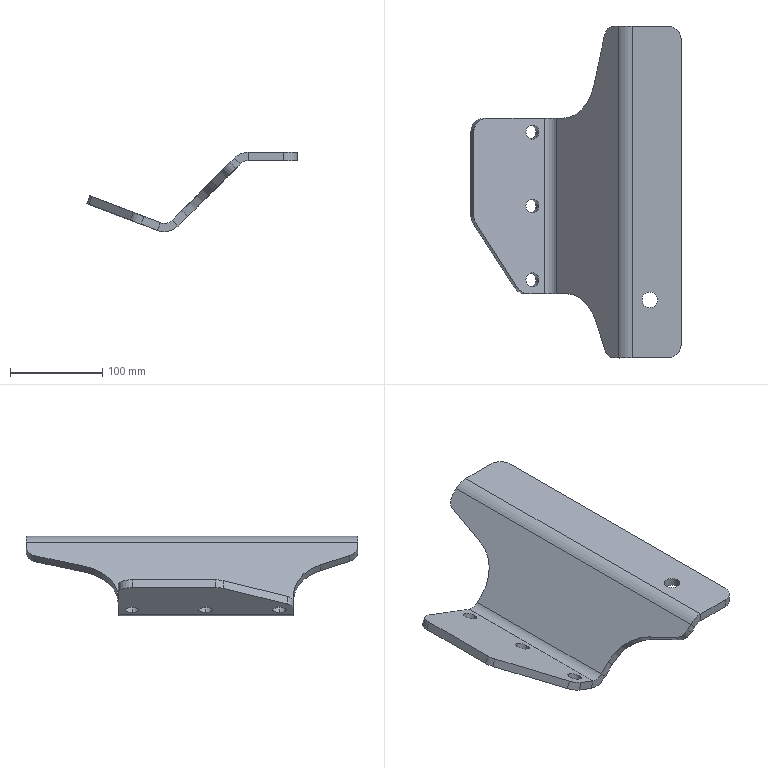Part | SolidWorks | features SM3dBend 2, FlatPattern 1, SMBaseFlange 1, SheetMetal 1 | 1 solid | 44 faces | box 228.191 x 360 x 86.08 mm | volume 576427 mm3 | plane 23 | cylinder 21 | commonest cylinder face diameters 30 x7 15 x6 17 x2 24 x2 42 x2 100 x2
STEP:
#1=CARTESIAN_POINT('',(-171.653,-115.,-77.046));
#2=VERTEX_POINT('',#1);
#3=CARTESIAN_POINT('',(-157.635,-115.,-82.385));
#4=VERTEX_POINT('',#3);
#5=CARTESIAN_POINT('',(-164.644,-115.,-79.716));
#6=DIRECTION('',(0.3559,0.,0.9345));
#7=DIRECTION('',(0.9345,0.,-0.3559));
#8=AXIS2_PLACEMENT_3D('',#5,#6,#7);
#9=CIRCLE('',#8,7.5);
#10=EDGE_CURVE('',#2,#4,#9,.T.);
#11=ORIENTED_EDGE('',*,*,#10,.F.);
#12=CARTESIAN_POINT('',(-168.45,-115.,-68.635));
#13=VERTEX_POINT('',#12);
#14=CARTESIAN_POINT('',(-171.653,-115.,-77.046));
#15=DIRECTION('',(0.3559,0.,0.9345));
#16=VECTOR('',#15,1000.);
#17=LINE('',#14,#16);
#18=EDGE_CURVE('',#2,#13,#17,.T.);
#19=ORIENTED_EDGE('',*,*,#18,.T.);
#20=CARTESIAN_POINT('',(-154.432,-115.,-73.974));
#21=VERTEX_POINT('',#20);
#22=CARTESIAN_POINT('',(-161.441,-115.,-71.305));
#23=DIRECTION('',(0.3559,0.,0.9345));
#24=DIRECTION('',(0.9345,0.,-0.3559));
#25=AXIS2_PLACEMENT_3D('',#22,#23,#24);
#26=CIRCLE('',#25,7.5);
#27=EDGE_CURVE('',#13,#21,#26,.T.);
#28=ORIENTED_EDGE('',*,*,#27,.T.);
#29=CARTESIAN_POINT('',(-157.635,-115.,-82.385));
#30=DIRECTION('',(0.3559,0.,0.9345));
#31=VECTOR('',#30,1000.);
#32=LINE('',#29,#31);
#33=EDGE_CURVE('',#4,#21,#32,.T.);
#34=ORIENTED_EDGE('',*,*,#33,.F.);
#35=EDGE_LOOP('',(#11,#19,#28,#34));
#36=FACE_OUTER_BOUND('',#35,.T.);
#37=CARTESIAN_POINT('',(-164.644,-115.,-79.716));
#38=DIRECTION('',(0.3559,0.,0.9345));
#39=DIRECTION('',(0.9345,0.,-0.3559));
#40=AXIS2_PLACEMENT_3D('',#37,#38,#39);
#41=CYLINDRICAL_SURFACE('',#40,7.5);
#42=ADVANCED_FACE('',(#36),#41,.F.);
#43=CARTESIAN_POINT('',(-171.653,-195.,-77.046));
#44=VERTEX_POINT('',#43);
#45=CARTESIAN_POINT('',(-157.635,-195.,-82.385));
#46=VERTEX_POINT('',#45);
#47=CARTESIAN_POINT('',(-164.644,-195.,-79.716));
#48=DIRECTION('',(0.3559,0.,0.9345));
#49=DIRECTION('',(0.9345,0.,-0.3559));
#50=AXIS2_PLACEMENT_3D('',#47,#48,#49);
#51=CIRCLE('',#50,7.5);
#52=EDGE_CURVE('',#44,#46,#51,.T.);
#53=ORIENTED_EDGE('',*,*,#52,.F.);
#54=CARTESIAN_POINT('',(-168.45,-195.,-68.635));
#55=VERTEX_POINT('',#54);
#56=CARTESIAN_POINT('',(-171.653,-195.,-77.046));
#57=DIRECTION('',(0.3559,0.,0.9345));
#58=VECTOR('',#57,1000.);
#59=LINE('',#56,#58);
#60=EDGE_CURVE('',#44,#55,#59,.T.);
#61=ORIENTED_EDGE('',*,*,#60,.T.);
#62=CARTESIAN_POINT('',(-154.432,-195.,-73.974));
#63=VERTEX_POINT('',#62);
#64=CARTESIAN_POINT('',(-161.441,-195.,-71.305));
#65=DIRECTION('',(0.3559,0.,0.9345));
#66=DIRECTION('',(0.9345,0.,-0.3559));
#67=AXIS2_PLACEMENT_3D('',#64,#65,#66);
#68=CIRCLE('',#67,7.5);
#69=EDGE_CURVE('',#55,#63,#68,.T.);
#70=ORIENTED_EDGE('',*,*,#69,.T.);
#71=CARTESIAN_POINT('',(-157.635,-195.,-82.385));
#72=DIRECTION('',(0.3559,0.,0.9345));
#73=VECTOR('',#72,1000.);
#74=LINE('',#71,#73);
#75=EDGE_CURVE('',#46,#63,#74,.T.);
#76=ORIENTED_EDGE('',*,*,#75,.F.);
#77=EDGE_LOOP('',(#53,#61,#70,#76));
#78=FACE_OUTER_BOUND('',#77,.T.);
#79=CARTESIAN_POINT('',(-164.644,-195.,-79.716));
#80=DIRECTION('',(0.3559,0.,0.9345));
#81=DIRECTION('',(0.9345,0.,-0.3559));
#82=AXIS2_PLACEMENT_3D('',#79,#80,#81);
#83=CYLINDRICAL_SURFACE('',#82,7.5);
#84=ADVANCED_FACE('',(#78),#83,.F.);
#85=CARTESIAN_POINT('',(-171.653,-275.,-77.046));
#86=VERTEX_POINT('',#85);
#87=CARTESIAN_POINT('',(-157.635,-275.,-82.385));
#88=VERTEX_POINT('',#87);
#89=CARTESIAN_POINT('',(-164.644,-275.,-79.716));
#90=DIRECTION('',(0.3559,0.,0.9345));
#91=DIRECTION('',(0.9345,0.,-0.3559));
#92=AXIS2_PLACEMENT_3D('',#89,#90,#91);
#93=CIRCLE('',#92,7.5);
#94=EDGE_CURVE('',#86,#88,#93,.T.);
#95=ORIENTED_EDGE('',*,*,#94,.F.);
#96=CARTESIAN_POINT('',(-168.45,-275.,-68.635));
#97=VERTEX_POINT('',#96);
#98=CARTESIAN_POINT('',(-171.653,-275.,-77.046));
#99=DIRECTION('',(0.3559,0.,0.9345));
#100=VECTOR('',#99,1000.);
#101=LINE('',#98,#100);
#102=EDGE_CURVE('',#86,#97,#101,.T.);
#103=ORIENTED_EDGE('',*,*,#102,.T.);
#104=CARTESIAN_POINT('',(-154.432,-275.,-73.974));
#105=VERTEX_POINT('',#104);
#106=CARTESIAN_POINT('',(-161.441,-275.,-71.305));
#107=DIRECTION('',(0.3559,0.,0.9345));
#108=DIRECTION('',(0.9345,0.,-0.3559));
#109=AXIS2_PLACEMENT_3D('',#106,#107,#108);
#110=CIRCLE('',#109,7.5);
#111=EDGE_CURVE('',#97,#105,#110,.T.);
#112=ORIENTED_EDGE('',*,*,#111,.T.);
#113=CARTESIAN_POINT('',(-157.635,-275.,-82.385));
#114=DIRECTION('',(0.3559,0.,0.9345));
#115=VECTOR('',#114,1000.);
#116=LINE('',#113,#115);
#117=EDGE_CURVE('',#88,#105,#116,.T.);
#118=ORIENTED_EDGE('',*,*,#117,.F.);
#119=EDGE_LOOP('',(#95,#103,#112,#118));
#120=FACE_OUTER_BOUND('',#119,.T.);
#121=CARTESIAN_POINT('',(-164.644,-275.,-79.716));
#122=DIRECTION('',(0.3559,0.,0.9345));
#123=DIRECTION('',(0.9345,0.,-0.3559));
#124=AXIS2_PLACEMENT_3D('',#121,#122,#123);
#125=CYLINDRICAL_SURFACE('',#124,7.5);
#126=ADVANCED_FACE('',(#120),#125,.F.);
#127=CARTESIAN_POINT('',(-42.5,-297.,-9.));
#128=VERTEX_POINT('',#127);
#129=CARTESIAN_POINT('',(-25.5,-297.,-9.));
#130=VERTEX_POINT('',#129);
#131=CARTESIAN_POINT('',(-34.,-297.,-9.));
#132=DIRECTION('',(0.,0.,1.));
#133=DIRECTION('',(1.,0.,0.));
#134=AXIS2_PLACEMENT_3D('',#131,#132,#133);
#135=CIRCLE('',#134,8.5);
#136=EDGE_CURVE('',#128,#130,#135,.T.);
#137=ORIENTED_EDGE('',*,*,#136,.F.);
#138=CARTESIAN_POINT('',(-42.5,-297.,0.));
#139=VERTEX_POINT('',#138);
#140=CARTESIAN_POINT('',(-42.5,-297.,-9.));
#141=DIRECTION('',(0.,0.,1.));
#142=VECTOR('',#141,1000.);
#143=LINE('',#140,#142);
#144=EDGE_CURVE('',#128,#139,#143,.T.);
#145=ORIENTED_EDGE('',*,*,#144,.T.);
#146=CARTESIAN_POINT('',(-25.5,-297.,0.));
#147=VERTEX_POINT('',#146);
#148=CARTESIAN_POINT('',(-34.,-297.,0.));
#149=DIRECTION('',(0.,0.,1.));
#150=DIRECTION('',(1.,0.,0.));
#151=AXIS2_PLACEMENT_3D('',#148,#149,#150);
#152=CIRCLE('',#151,8.5);
#153=EDGE_CURVE('',#139,#147,#152,.T.);
#154=ORIENTED_EDGE('',*,*,#153,.T.);
#155=CARTESIAN_POINT('',(-25.5,-297.,-9.));
#156=DIRECTION('',(0.,0.,1.));
#157=VECTOR('',#156,1000.);
#158=LINE('',#155,#157);
#159=EDGE_CURVE('',#130,#147,#158,.T.);
#160=ORIENTED_EDGE('',*,*,#159,.F.);
#161=EDGE_LOOP('',(#137,#145,#154,#160));
#162=FACE_OUTER_BOUND('',#161,.T.);
#163=CARTESIAN_POINT('',(-34.,-297.,-9.));
#164=DIRECTION('',(0.,0.,1.));
#165=DIRECTION('',(1.,0.,0.));
#166=AXIS2_PLACEMENT_3D('',#163,#164,#165);
#167=CYLINDRICAL_SURFACE('',#166,8.5);
#168=ADVANCED_FACE('',(#162),#167,.F.);
#169=CARTESIAN_POINT('',(-129.22,-290.,-79.929));
#170=VERTEX_POINT('',#169);
#171=CARTESIAN_POINT('',(-118.776,-290.,-69.485));
#172=VERTEX_POINT('',#171);
#173=CARTESIAN_POINT('',(-156.155,-290.,-106.864));
#174=DIRECTION('',(0.7071,0.,0.7071));
#175=VECTOR('',#174,1000.);
#176=LINE('',#173,#175);
#177=EDGE_CURVE('',#170,#172,#176,.T.);
#178=ORIENTED_EDGE('',*,*,#177,.F.);
#179=CARTESIAN_POINT('',(-129.22,-100.,-79.929));
#180=VERTEX_POINT('',#179);
#181=CARTESIAN_POINT('',(-129.22,-345.,-79.929));
#182=DIRECTION('',(0.,1.,0.));
#183=VECTOR('',#182,1000.);
#184=LINE('',#181,#183);
#185=EDGE_CURVE('',#170,#180,#184,.T.);
#186=ORIENTED_EDGE('',*,*,#185,.T.);
#187=CARTESIAN_POINT('',(-122.208,-100.,-72.917));
#188=VERTEX_POINT('',#187);
#189=CARTESIAN_POINT('',(-122.208,-100.,-72.917));
#190=DIRECTION('',(-0.7071,0.,-0.7071));
#191=VECTOR('',#190,1000.);
#192=LINE('',#189,#191);
#193=EDGE_CURVE('',#188,#180,#192,.T.);
#194=ORIENTED_EDGE('',*,*,#193,.F.);
#195=CARTESIAN_POINT('',(-88.344,-64.367,-39.053));
#196=VERTEX_POINT('',#195);
#197=CARTESIAN_POINT('',(-122.208,-50.,-72.917));
#198=DIRECTION('',(0.7071,0.,-0.7071));
#199=DIRECTION('',(-0.7071,0.,-0.7071));
#200=AXIS2_PLACEMENT_3D('',#197,#198,#199);
#201=CIRCLE('',#200,50.);
#202=EDGE_CURVE('',#196,#188,#201,.T.);
#203=ORIENTED_EDGE('',*,*,#202,.F.);
#204=CARTESIAN_POINT('',(-76.957,-10.69,-27.666));
#205=VERTEX_POINT('',#204);
#206=CARTESIAN_POINT('',(-76.957,-10.69,-27.666));
#207=DIRECTION('',(-0.2032,-0.9578,-0.2032));
#208=VECTOR('',#207,1000.);
#209=LINE('',#206,#208);
#210=EDGE_CURVE('',#205,#196,#209,.T.);
#211=ORIENTED_EDGE('',*,*,#210,.F.);
#212=CARTESIAN_POINT('',(-66.798,0.,-17.507));
#213=VERTEX_POINT('',#212);
#214=CARTESIAN_POINT('',(-66.798,-15.,-17.507));
#215=DIRECTION('',(-0.7071,0.,0.7071));
#216=DIRECTION('',(0.7071,0.,0.7071));
#217=AXIS2_PLACEMENT_3D('',#214,#215,#216);
#218=CIRCLE('',#217,15.);
#219=EDGE_CURVE('',#213,#205,#218,.T.);
#220=ORIENTED_EDGE('',*,*,#219,.F.);
#221=CARTESIAN_POINT('',(-61.806,0.,-12.515));
#222=VERTEX_POINT('',#221);
#223=CARTESIAN_POINT('',(-25.546,0.,23.745));
#224=DIRECTION('',(-0.7071,0.,-0.7071));
#225=VECTOR('',#224,1000.);
#226=LINE('',#223,#225);
#227=EDGE_CURVE('',#222,#213,#226,.T.);
#228=ORIENTED_EDGE('',*,*,#227,.F.);
#229=CARTESIAN_POINT('',(-61.806,-360.,-12.515));
#230=VERTEX_POINT('',#229);
#231=CARTESIAN_POINT('',(-61.806,-345.,-12.515));
#232=DIRECTION('',(0.,-1.,0.));
#233=VECTOR('',#232,1000.);
#234=LINE('',#231,#233);
#235=EDGE_CURVE('',#222,#230,#234,.T.);
#236=ORIENTED_EDGE('',*,*,#235,.T.);
#237=CARTESIAN_POINT('',(-66.798,-360.,-17.507));
#238=VERTEX_POINT('',#237);
#239=CARTESIAN_POINT('',(-66.798,-360.,-17.507));
#240=DIRECTION('',(0.7071,0.,0.7071));
#241=VECTOR('',#240,1000.);
#242=LINE('',#239,#241);
#243=EDGE_CURVE('',#238,#230,#242,.T.);
#244=ORIENTED_EDGE('',*,*,#243,.F.);
#245=CARTESIAN_POINT('',(-76.473,-351.148,-27.182));
#246=VERTEX_POINT('',#245);
#247=CARTESIAN_POINT('',(-66.798,-345.,-17.507));
#248=DIRECTION('',(-0.7071,0.,0.7071));
#249=DIRECTION('',(0.7071,0.,0.7071));
#250=AXIS2_PLACEMENT_3D('',#247,#248,#249);
#251=CIRCLE('',#250,15.);
#252=EDGE_CURVE('',#246,#238,#251,.T.);
#253=ORIENTED_EDGE('',*,*,#252,.F.);
#254=CARTESIAN_POINT('',(-86.527,-319.506,-37.236));
#255=VERTEX_POINT('',#254);
#256=CARTESIAN_POINT('',(-86.527,-319.506,-37.236));
#257=DIRECTION('',(0.2898,-0.9121,0.2898));
#258=VECTOR('',#257,1000.);
#259=LINE('',#256,#258);
#260=EDGE_CURVE('',#255,#246,#259,.T.);
#261=ORIENTED_EDGE('',*,*,#260,.F.);
#262=CARTESIAN_POINT('',(-118.776,-340.,-69.485));
#263=DIRECTION('',(0.7071,0.,-0.7071));
#264=DIRECTION('',(-0.7071,0.,-0.7071));
#265=AXIS2_PLACEMENT_3D('',#262,#263,#264);
#266=CIRCLE('',#265,50.);
#267=EDGE_CURVE('',#172,#255,#266,.T.);
#268=ORIENTED_EDGE('',*,*,#267,.F.);
#269=EDGE_LOOP('',(#178,#186,#194,#203,#211,#220,#228,#236,#244,#253,#261,#268));
#270=FACE_OUTER_BOUND('',#269,.T.);
#271=CARTESIAN_POINT('',(-66.798,-345.,-17.507));
#272=DIRECTION('',(-0.7071,0.,0.7071));
#273=DIRECTION('',(0.7071,0.,0.7071));
#274=AXIS2_PLACEMENT_3D('',#271,#272,#273);
#275=PLANE('',#274);
#276=ADVANCED_FACE('',(#270),#275,.F.);
#277=CARTESIAN_POINT('',(-82.837,-351.148,-20.818));
#278=VERTEX_POINT('',#277);
#279=CARTESIAN_POINT('',(-73.162,-360.,-11.143));
#280=VERTEX_POINT('',#279);
#281=CARTESIAN_POINT('',(-73.162,-345.,-11.143));
#282=DIRECTION('',(-0.7071,0.,0.7071));
#283=DIRECTION('',(0.7071,0.,0.7071));
#284=AXIS2_PLACEMENT_3D('',#281,#282,#283);
#285=CIRCLE('',#284,15.);
#286=EDGE_CURVE('',#278,#280,#285,.T.);
#287=ORIENTED_EDGE('',*,*,#286,.F.);
#288=CARTESIAN_POINT('',(-76.473,-351.148,-27.182));
#289=DIRECTION('',(-0.7071,0.,0.7071));
#290=VECTOR('',#289,1000.);
#291=LINE('',#288,#290);
#292=EDGE_CURVE('',#246,#278,#291,.T.);
#293=ORIENTED_EDGE('',*,*,#292,.F.);
#294=ORIENTED_EDGE('',*,*,#252,.T.);
#295=CARTESIAN_POINT('',(-66.798,-360.,-17.507));
#296=DIRECTION('',(-0.7071,0.,0.7071));
#297=VECTOR('',#296,1000.);
#298=LINE('',#295,#297);
#299=EDGE_CURVE('',#238,#280,#298,.T.);
#300=ORIENTED_EDGE('',*,*,#299,.T.);
#301=EDGE_LOOP('',(#287,#293,#294,#300));
#302=FACE_OUTER_BOUND('',#301,.T.);
#303=CARTESIAN_POINT('',(-66.798,-345.,-17.507));
#304=DIRECTION('',(-0.7071,0.,0.7071));
#305=DIRECTION('',(0.7071,0.,0.7071));
#306=AXIS2_PLACEMENT_3D('',#303,#304,#305);
#307=CYLINDRICAL_SURFACE('',#306,15.);
#308=ADVANCED_FACE('',(#302),#307,.T.);
#309=CARTESIAN_POINT('',(-92.891,-319.506,-30.872));
#310=VERTEX_POINT('',#309);
#311=CARTESIAN_POINT('',(-92.891,-319.506,-30.872));
#312=DIRECTION('',(0.2898,-0.9121,0.2898));
#313=VECTOR('',#312,1000.);
#314=LINE('',#311,#313);
#315=EDGE_CURVE('',#310,#278,#314,.T.);
#316=ORIENTED_EDGE('',*,*,#315,.F.);
#317=CARTESIAN_POINT('',(-86.527,-319.506,-37.236));
#318=DIRECTION('',(-0.7071,0.,0.7071));
#319=VECTOR('',#318,1000.);
#320=LINE('',#317,#319);
#321=EDGE_CURVE('',#255,#310,#320,.T.);
#322=ORIENTED_EDGE('',*,*,#321,.F.);
#323=ORIENTED_EDGE('',*,*,#260,.T.);
#324=ORIENTED_EDGE('',*,*,#292,.T.);
#325=EDGE_LOOP('',(#316,#322,#323,#324));
#326=FACE_OUTER_BOUND('',#325,.T.);
#327=CARTESIAN_POINT('',(-86.527,-319.506,-37.236));
#328=DIRECTION('',(-0.645,-0.4099,-0.645));
#329=DIRECTION('',(0.2898,-0.9121,0.2898));
#330=AXIS2_PLACEMENT_3D('',#327,#328,#329);
#331=PLANE('',#330);
#332=ADVANCED_FACE('',(#326),#331,.T.);
#333=CARTESIAN_POINT('',(-125.14,-290.,-63.121));
#334=VERTEX_POINT('',#333);
#335=CARTESIAN_POINT('',(-125.14,-340.,-63.121));
#336=DIRECTION('',(0.7071,0.,-0.7071));
#337=DIRECTION('',(-0.7071,0.,-0.7071));
#338=AXIS2_PLACEMENT_3D('',#335,#336,#337);
#339=CIRCLE('',#338,50.);
#340=EDGE_CURVE('',#334,#310,#339,.T.);
#341=ORIENTED_EDGE('',*,*,#340,.F.);
#342=CARTESIAN_POINT('',(-118.776,-290.,-69.485));
#343=DIRECTION('',(-0.7071,0.,0.7071));
#344=VECTOR('',#343,1000.);
#345=LINE('',#342,#344);
#346=EDGE_CURVE('',#172,#334,#345,.T.);
#347=ORIENTED_EDGE('',*,*,#346,.F.);
#348=ORIENTED_EDGE('',*,*,#267,.T.);
#349=ORIENTED_EDGE('',*,*,#321,.T.);
#350=EDGE_LOOP('',(#341,#347,#348,#349));
#351=FACE_OUTER_BOUND('',#350,.T.);
#352=CARTESIAN_POINT('',(-118.776,-340.,-69.485));
#353=DIRECTION('',(-0.7071,0.,0.7071));
#354=DIRECTION('',(0.7071,0.,0.7071));
#355=AXIS2_PLACEMENT_3D('',#352,#353,#354);
#356=CYLINDRICAL_SURFACE('',#355,50.);
#357=ADVANCED_FACE('',(#351),#356,.F.);
#358=CARTESIAN_POINT('',(-135.584,-290.,-73.565));
#359=VERTEX_POINT('',#358);
#360=CARTESIAN_POINT('',(-129.22,-290.,-79.929));
#361=DIRECTION('',(-0.7071,0.,0.7071));
#362=VECTOR('',#361,1000.);
#363=LINE('',#360,#362);
#364=EDGE_CURVE('',#170,#359,#363,.T.);
#365=ORIENTED_EDGE('',*,*,#364,.F.);
#366=ORIENTED_EDGE('',*,*,#177,.T.);
#367=ORIENTED_EDGE('',*,*,#346,.T.);
#368=CARTESIAN_POINT('',(-162.519,-290.,-100.5));
#369=DIRECTION('',(0.7071,0.,0.7071));
#370=VECTOR('',#369,1000.);
#371=LINE('',#368,#370);
#372=EDGE_CURVE('',#359,#334,#371,.T.);
#373=ORIENTED_EDGE('',*,*,#372,.F.);
#374=EDGE_LOOP('',(#365,#366,#367,#373));
#375=FACE_OUTER_BOUND('',#374,.T.);
#376=CARTESIAN_POINT('',(-156.155,-290.,-106.864));
#377=DIRECTION('',(0.,-1.,0.));
#378=DIRECTION('',(0.7071,0.,0.7071));
#379=AXIS2_PLACEMENT_3D('',#376,#377,#378);
#380=PLANE('',#379);
#381=ADVANCED_FACE('',(#375),#380,.T.);
#382=CARTESIAN_POINT('',(-135.584,-100.,-73.565));
#383=VERTEX_POINT('',#382);
#384=CARTESIAN_POINT('',(-129.22,-100.,-79.929));
#385=DIRECTION('',(0.7071,0.,-0.7071));
#386=VECTOR('',#385,1000.);
#387=LINE('',#384,#386);
#388=EDGE_CURVE('',#383,#180,#387,.T.);
#389=ORIENTED_EDGE('',*,*,#388,.F.);
#390=CARTESIAN_POINT('',(-128.572,-100.,-66.553));
#391=VERTEX_POINT('',#390);
#392=CARTESIAN_POINT('',(-128.572,-100.,-66.553));
#393=DIRECTION('',(-0.7071,0.,-0.7071));
#394=VECTOR('',#393,1000.);
#395=LINE('',#392,#394);
#396=EDGE_CURVE('',#391,#383,#395,.T.);
#397=ORIENTED_EDGE('',*,*,#396,.F.);
#398=CARTESIAN_POINT('',(-122.208,-100.,-72.917));
#399=DIRECTION('',(-0.7071,0.,0.7071));
#400=VECTOR('',#399,1000.);
#401=LINE('',#398,#400);
#402=EDGE_CURVE('',#188,#391,#401,.T.);
#403=ORIENTED_EDGE('',*,*,#402,.F.);
#404=ORIENTED_EDGE('',*,*,#193,.T.);
#405=EDGE_LOOP('',(#389,#397,#403,#404));
#406=FACE_OUTER_BOUND('',#405,.T.);
#407=CARTESIAN_POINT('',(-122.208,-100.,-72.917));
#408=DIRECTION('',(0.,1.,0.));
#409=DIRECTION('',(-0.7071,0.,-0.7071));
#410=AXIS2_PLACEMENT_3D('',#407,#408,#409);
#411=PLANE('',#410);
#412=ADVANCED_FACE('',(#406),#411,.T.);
#413=CARTESIAN_POINT('',(-94.708,-64.367,-32.689));
#414=VERTEX_POINT('',#413);
#415=CARTESIAN_POINT('',(-128.572,-50.,-66.553));
#416=DIRECTION('',(0.7071,0.,-0.7071));
#417=DIRECTION('',(-0.7071,0.,-0.7071));
#418=AXIS2_PLACEMENT_3D('',#415,#416,#417);
#419=CIRCLE('',#418,50.);
#420=EDGE_CURVE('',#414,#391,#419,.T.);
#421=ORIENTED_EDGE('',*,*,#420,.F.);
#422=CARTESIAN_POINT('',(-88.344,-64.367,-39.053));
#423=DIRECTION('',(-0.7071,0.,0.7071));
#424=VECTOR('',#423,1000.);
#425=LINE('',#422,#424);
#426=EDGE_CURVE('',#196,#414,#425,.T.);
#427=ORIENTED_EDGE('',*,*,#426,.F.);
#428=ORIENTED_EDGE('',*,*,#202,.T.);
#429=ORIENTED_EDGE('',*,*,#402,.T.);
#430=EDGE_LOOP('',(#421,#427,#428,#429));
#431=FACE_OUTER_BOUND('',#430,.T.);
#432=CARTESIAN_POINT('',(-122.208,-50.,-72.917));
#433=DIRECTION('',(-0.7071,0.,0.7071));
#434=DIRECTION('',(0.7071,0.,0.7071));
#435=AXIS2_PLACEMENT_3D('',#432,#433,#434);
#436=CYLINDRICAL_SURFACE('',#435,50.);
#437=ADVANCED_FACE('',(#431),#436,.F.);
#438=CARTESIAN_POINT('',(-83.321,-10.69,-21.302));
#439=VERTEX_POINT('',#438);
#440=CARTESIAN_POINT('',(-83.321,-10.69,-21.302));
#441=DIRECTION('',(-0.2032,-0.9578,-0.2032));
#442=VECTOR('',#441,1000.);
#443=LINE('',#440,#442);
#444=EDGE_CURVE('',#439,#414,#443,.T.);
#445=ORIENTED_EDGE('',*,*,#444,.F.);
#446=CARTESIAN_POINT('',(-76.957,-10.69,-27.666));
#447=DIRECTION('',(-0.7071,0.,0.7071));
#448=VECTOR('',#447,1000.);
#449=LINE('',#446,#448);
#450=EDGE_CURVE('',#205,#439,#449,.T.);
#451=ORIENTED_EDGE('',*,*,#450,.F.);
#452=ORIENTED_EDGE('',*,*,#210,.T.);
#453=ORIENTED_EDGE('',*,*,#426,.T.);
#454=EDGE_LOOP('',(#445,#451,#452,#453));
#455=FACE_OUTER_BOUND('',#454,.T.);
#456=CARTESIAN_POINT('',(-76.957,-10.69,-27.666));
#457=DIRECTION('',(-0.6773,0.2873,-0.6773));
#458=DIRECTION('',(-0.2032,-0.9578,-0.2032));
#459=AXIS2_PLACEMENT_3D('',#456,#457,#458);
#460=PLANE('',#459);
#461=ADVANCED_FACE('',(#455),#460,.T.);
#462=CARTESIAN_POINT('',(-73.162,0.,-11.143));
#463=VERTEX_POINT('',#462);
#464=CARTESIAN_POINT('',(-73.162,-15.,-11.143));
#465=DIRECTION('',(-0.7071,0.,0.7071));
#466=DIRECTION('',(0.7071,0.,0.7071));
#467=AXIS2_PLACEMENT_3D('',#464,#465,#466);
#468=CIRCLE('',#467,15.);
#469=EDGE_CURVE('',#463,#439,#468,.T.);
#470=ORIENTED_EDGE('',*,*,#469,.F.);
#471=CARTESIAN_POINT('',(-66.798,0.,-17.507));
#472=DIRECTION('',(-0.7071,0.,0.7071));
#473=VECTOR('',#472,1000.);
#474=LINE('',#471,#473);
#475=EDGE_CURVE('',#213,#463,#474,.T.);
#476=ORIENTED_EDGE('',*,*,#475,.F.);
#477=ORIENTED_EDGE('',*,*,#219,.T.);
#478=ORIENTED_EDGE('',*,*,#450,.T.);
#479=EDGE_LOOP('',(#470,#476,#477,#478));
#480=FACE_OUTER_BOUND('',#479,.T.);
#481=CARTESIAN_POINT('',(-66.798,-15.,-17.507));
#482=DIRECTION('',(-0.7071,0.,0.7071));
#483=DIRECTION('',(0.7071,0.,0.7071));
#484=AXIS2_PLACEMENT_3D('',#481,#482,#483);
#485=CYLINDRICAL_SURFACE('',#484,15.);
#486=ADVANCED_FACE('',(#480),#485,.T.);
#487=CARTESIAN_POINT('',(-68.17,0.,-6.151));
#488=VERTEX_POINT('',#487);
#489=CARTESIAN_POINT('',(-61.806,0.,-12.515));
#490=DIRECTION('',(-0.7071,0.,0.7071));
#491=VECTOR('',#490,1000.);
#492=LINE('',#489,#491);
#493=EDGE_CURVE('',#222,#488,#492,.T.);
#494=ORIENTED_EDGE('',*,*,#493,.F.);
#495=ORIENTED_EDGE('',*,*,#227,.T.);
#496=ORIENTED_EDGE('',*,*,#475,.T.);
#497=CARTESIAN_POINT('',(-31.91,0.,30.109));
#498=DIRECTION('',(-0.7071,0.,-0.7071));
#499=VECTOR('',#498,1000.);
#500=LINE('',#497,#499);
#501=EDGE_CURVE('',#488,#463,#500,.T.);
#502=ORIENTED_EDGE('',*,*,#501,.F.);
#503=EDGE_LOOP('',(#494,#495,#496,#502));
#504=FACE_OUTER_BOUND('',#503,.T.);
#505=CARTESIAN_POINT('',(-25.546,0.,23.745));
#506=DIRECTION('',(0.,1.,0.));
#507=DIRECTION('',(-0.7071,0.,0.7071));
#508=AXIS2_PLACEMENT_3D('',#505,#506,#507);
#509=PLANE('',#508);
#510=ADVANCED_FACE('',(#504),#509,.T.);
#511=CARTESIAN_POINT('',(-68.17,-360.,-6.151));
#512=VERTEX_POINT('',#511);
#513=CARTESIAN_POINT('',(-61.806,-360.,-12.515));
#514=DIRECTION('',(0.7071,0.,-0.7071));
#515=VECTOR('',#514,1000.);
#516=LINE('',#513,#515);
#517=EDGE_CURVE('',#512,#230,#516,.T.);
#518=ORIENTED_EDGE('',*,*,#517,.F.);
#519=CARTESIAN_POINT('',(-73.162,-360.,-11.143));
#520=DIRECTION('',(0.7071,0.,0.7071));
#521=VECTOR('',#520,1000.);
#522=LINE('',#519,#521);
#523=EDGE_CURVE('',#280,#512,#522,.T.);
#524=ORIENTED_EDGE('',*,*,#523,.F.);
#525=ORIENTED_EDGE('',*,*,#299,.F.);
#526=ORIENTED_EDGE('',*,*,#243,.T.);
#527=EDGE_LOOP('',(#518,#524,#525,#526));
#528=FACE_OUTER_BOUND('',#527,.T.);
#529=CARTESIAN_POINT('',(-66.798,-360.,-17.507));
#530=DIRECTION('',(0.,-1.,0.));
#531=DIRECTION('',(0.7071,0.,0.7071));
#532=AXIS2_PLACEMENT_3D('',#529,#530,#531);
#533=PLANE('',#532);
#534=ADVANCED_FACE('',(#528),#533,.T.);
#535=CARTESIAN_POINT('',(-135.584,-345.,-73.565));
#536=DIRECTION('',(0.,1.,0.));
#537=VECTOR('',#536,1000.);
#538=LINE('',#535,#537);
#539=EDGE_CURVE('',#359,#383,#538,.T.);
#540=ORIENTED_EDGE('',*,*,#539,.F.);
#541=ORIENTED_EDGE('',*,*,#372,.T.);
#542=ORIENTED_EDGE('',*,*,#340,.T.);
#543=ORIENTED_EDGE('',*,*,#315,.T.);
#544=ORIENTED_EDGE('',*,*,#286,.T.);
#545=ORIENTED_EDGE('',*,*,#523,.T.);
#546=CARTESIAN_POINT('',(-68.17,-345.,-6.151));
#547=DIRECTION('',(0.,-1.,0.));
#548=VECTOR('',#547,1000.);
#549=LINE('',#546,#548);
#550=EDGE_CURVE('',#488,#512,#549,.T.);
#551=ORIENTED_EDGE('',*,*,#550,.F.);
#552=ORIENTED_EDGE('',*,*,#501,.T.);
#553=ORIENTED_EDGE('',*,*,#469,.T.);
#554=ORIENTED_EDGE('',*,*,#444,.T.);
#555=ORIENTED_EDGE('',*,*,#420,.T.);
#556=ORIENTED_EDGE('',*,*,#396,.T.);
#557=EDGE_LOOP('',(#540,#541,#542,#543,#544,#545,#551,#552,#553,#554,#555,#556));
#558=FACE_OUTER_BOUND('',#557,.T.);
#559=CARTESIAN_POINT('',(-73.162,-345.,-11.143));
#560=DIRECTION('',(-0.7071,0.,0.7071));
#561=DIRECTION('',(0.7071,0.,0.7071));
#562=AXIS2_PLACEMENT_3D('',#559,#560,#561);
#563=PLANE('',#562);
#564=ADVANCED_FACE('',(#558),#563,.T.);
#565=ORIENTED_EDGE('',*,*,#144,.F.);
#566=CARTESIAN_POINT('',(-34.,-297.,-9.));
#567=DIRECTION('',(0.,0.,1.));
#568=DIRECTION('',(1.,0.,0.));
#569=AXIS2_PLACEMENT_3D('',#566,#567,#568);
#570=CIRCLE('',#569,8.5);
#571=EDGE_CURVE('',#130,#128,#570,.T.);
#572=ORIENTED_EDGE('',*,*,#571,.F.);
#573=ORIENTED_EDGE('',*,*,#159,.T.);
#574=CARTESIAN_POINT('',(-34.,-297.,0.));
#575=DIRECTION('',(0.,0.,1.));
#576=DIRECTION('',(1.,0.,0.));
#577=AXIS2_PLACEMENT_3D('',#574,#575,#576);
#578=CIRCLE('',#577,8.5);
#579=EDGE_CURVE('',#147,#139,#578,.T.);
#580=ORIENTED_EDGE('',*,*,#579,.T.);
#581=EDGE_LOOP('',(#565,#572,#573,#580));
#582=FACE_OUTER_BOUND('',#581,.T.);
#583=CARTESIAN_POINT('',(-34.,-297.,-9.));
#584=DIRECTION('',(0.,0.,1.));
#585=DIRECTION('',(1.,0.,0.));
#586=AXIS2_PLACEMENT_3D('',#583,#584,#585);
#587=CYLINDRICAL_SURFACE('',#586,8.5);
#588=ADVANCED_FACE('',(#582),#587,.F.);
#589=CARTESIAN_POINT('',(-15.,-360.,0.));
#590=VERTEX_POINT('',#589);
#591=CARTESIAN_POINT('',(0.,-345.,0.));
#592=VERTEX_POINT('',#591);
#593=CARTESIAN_POINT('',(-15.,-345.,0.));
#594=DIRECTION('',(0.,0.,1.));
#595=DIRECTION('',(1.,0.,0.));
#596=AXIS2_PLACEMENT_3D('',#593,#594,#595);
#597=CIRCLE('',#596,15.);
#598=EDGE_CURVE('',#590,#592,#597,.T.);
#599=ORIENTED_EDGE('',*,*,#598,.F.);
#600=CARTESIAN_POINT('',(-15.,-360.,-9.));
#601=VERTEX_POINT('',#600);
#602=CARTESIAN_POINT('',(-15.,-360.,-9.));
#603=DIRECTION('',(0.,0.,1.));
#604=VECTOR('',#603,1000.);
#605=LINE('',#602,#604);
#606=EDGE_CURVE('',#601,#590,#605,.T.);
#607=ORIENTED_EDGE('',*,*,#606,.F.);
#608=CARTESIAN_POINT('',(0.,-345.,-9.));
#609=VERTEX_POINT('',#608);
#610=CARTESIAN_POINT('',(-15.,-345.,-9.));
#611=DIRECTION('',(0.,0.,1.));
#612=DIRECTION('',(1.,0.,0.));
#613=AXIS2_PLACEMENT_3D('',#610,#611,#612);
#614=CIRCLE('',#613,15.);
#615=EDGE_CURVE('',#601,#609,#614,.T.);
#616=ORIENTED_EDGE('',*,*,#615,.T.);
#617=CARTESIAN_POINT('',(0.,-345.,-9.));
#618=DIRECTION('',(0.,0.,1.));
#619=VECTOR('',#618,1000.);
#620=LINE('',#617,#619);
#621=EDGE_CURVE('',#609,#592,#620,.T.);
#622=ORIENTED_EDGE('',*,*,#621,.T.);
#623=EDGE_LOOP('',(#599,#607,#616,#622));
#624=FACE_OUTER_BOUND('',#623,.T.);
#625=CARTESIAN_POINT('',(-15.,-345.,-9.));
#626=DIRECTION('',(0.,0.,1.));
#627=DIRECTION('',(1.,0.,0.));
#628=AXIS2_PLACEMENT_3D('',#625,#626,#627);
#629=CYLINDRICAL_SURFACE('',#628,15.);
#630=ADVANCED_FACE('',(#624),#629,.T.);
#631=CARTESIAN_POINT('',(0.,-15.,0.));
#632=VERTEX_POINT('',#631);
#633=CARTESIAN_POINT('',(0.,-345.,0.));
#634=DIRECTION('',(0.,1.,0.));
#635=VECTOR('',#634,1000.);
#636=LINE('',#633,#635);
#637=EDGE_CURVE('',#592,#632,#636,.T.);
#638=ORIENTED_EDGE('',*,*,#637,.F.);
#639=ORIENTED_EDGE('',*,*,#621,.F.);
#640=CARTESIAN_POINT('',(0.,-15.,-9.));
#641=VERTEX_POINT('',#640);
#642=CARTESIAN_POINT('',(0.,-345.,-9.));
#643=DIRECTION('',(0.,1.,0.));
#644=VECTOR('',#643,1000.);
#645=LINE('',#642,#644);
#646=EDGE_CURVE('',#609,#641,#645,.T.);
#647=ORIENTED_EDGE('',*,*,#646,.T.);
#648=CARTESIAN_POINT('',(0.,-15.,-9.));
#649=DIRECTION('',(0.,0.,1.));
#650=VECTOR('',#649,1000.);
#651=LINE('',#648,#650);
#652=EDGE_CURVE('',#641,#632,#651,.T.);
#653=ORIENTED_EDGE('',*,*,#652,.T.);
#654=EDGE_LOOP('',(#638,#639,#647,#653));
#655=FACE_OUTER_BOUND('',#654,.T.);
#656=CARTESIAN_POINT('',(0.,-345.,-9.));
#657=DIRECTION('',(1.,0.,0.));
#658=DIRECTION('',(0.,0.,-1.));
#659=AXIS2_PLACEMENT_3D('',#656,#657,#658);
#660=PLANE('',#659);
#661=ADVANCED_FACE('',(#655),#660,.T.);
#662=CARTESIAN_POINT('',(-15.,0.,0.));
#663=VERTEX_POINT('',#662);
#664=CARTESIAN_POINT('',(-15.,-15.,0.));
#665=DIRECTION('',(0.,0.,1.));
#666=DIRECTION('',(-1.,0.,0.));
#667=AXIS2_PLACEMENT_3D('',#664,#665,#666);
#668=CIRCLE('',#667,15.);
#669=EDGE_CURVE('',#632,#663,#668,.T.);
#670=ORIENTED_EDGE('',*,*,#669,.F.);
#671=ORIENTED_EDGE('',*,*,#652,.F.);
#672=CARTESIAN_POINT('',(-15.,0.,-9.));
#673=VERTEX_POINT('',#672);
#674=CARTESIAN_POINT('',(-15.,-15.,-9.));
#675=DIRECTION('',(0.,0.,1.));
#676=DIRECTION('',(-1.,0.,0.));
#677=AXIS2_PLACEMENT_3D('',#674,#675,#676);
#678=CIRCLE('',#677,15.);
#679=EDGE_CURVE('',#641,#673,#678,.T.);
#680=ORIENTED_EDGE('',*,*,#679,.T.);
#681=CARTESIAN_POINT('',(-15.,0.,-9.));
#682=DIRECTION('',(0.,0.,1.));
#683=VECTOR('',#682,1000.);
#684=LINE('',#681,#683);
#685=EDGE_CURVE('',#673,#663,#684,.T.);
#686=ORIENTED_EDGE('',*,*,#685,.T.);
#687=EDGE_LOOP('',(#670,#671,#680,#686));
#688=FACE_OUTER_BOUND('',#687,.T.);
#689=CARTESIAN_POINT('',(-15.,-15.,-9.));
#690=DIRECTION('',(0.,0.,1.));
#691=DIRECTION('',(1.,0.,0.));
#692=AXIS2_PLACEMENT_3D('',#689,#690,#691);
#693=CYLINDRICAL_SURFACE('',#692,15.);
#694=ADVANCED_FACE('',(#688),#693,.T.);
#695=CARTESIAN_POINT('',(-53.32,0.,-9.));
#696=VERTEX_POINT('',#695);
#697=CARTESIAN_POINT('',(-53.32,-360.,-9.));
#698=VERTEX_POINT('',#697);
#699=CARTESIAN_POINT('',(-53.32,-345.,-9.));
#700=DIRECTION('',(0.,-1.,0.));
#701=VECTOR('',#700,1000.);
#702=LINE('',#699,#701);
#703=EDGE_CURVE('',#696,#698,#702,.T.);
#704=ORIENTED_EDGE('',*,*,#703,.F.);
#705=CARTESIAN_POINT('',(-15.,0.,-9.));
#706=DIRECTION('',(-1.,0.,0.));
#707=VECTOR('',#706,1000.);
#708=LINE('',#705,#707);
#709=EDGE_CURVE('',#673,#696,#708,.T.);
#710=ORIENTED_EDGE('',*,*,#709,.F.);
#711=ORIENTED_EDGE('',*,*,#679,.F.);
#712=ORIENTED_EDGE('',*,*,#646,.F.);
#713=ORIENTED_EDGE('',*,*,#615,.F.);
#714=CARTESIAN_POINT('',(-73.34,-360.,-9.));
#715=DIRECTION('',(1.,0.,0.));
#716=VECTOR('',#715,1000.);
#717=LINE('',#714,#716);
#718=EDGE_CURVE('',#698,#601,#717,.T.);
#719=ORIENTED_EDGE('',*,*,#718,.F.);
#720=EDGE_LOOP('',(#704,#710,#711,#712,#713,#719));
#721=FACE_OUTER_BOUND('',#720,.T.);
#722=ORIENTED_EDGE('',*,*,#571,.T.);
#723=ORIENTED_EDGE('',*,*,#136,.T.);
#724=EDGE_LOOP('',(#722,#723));
#725=FACE_BOUND('',#724,.T.);
#726=CARTESIAN_POINT('',(-73.34,-345.,-9.));
#727=DIRECTION('',(0.,0.,1.));
#728=DIRECTION('',(1.,0.,0.));
#729=AXIS2_PLACEMENT_3D('',#726,#727,#728);
#730=PLANE('',#729);
#731=ADVANCED_FACE('',(#721,#725),#730,.F.);
#732=ORIENTED_EDGE('',*,*,#709,.T.);
#733=CARTESIAN_POINT('',(-53.32,0.,0.));
#734=VERTEX_POINT('',#733);
#735=CARTESIAN_POINT('',(-53.32,0.,-9.));
#736=DIRECTION('',(0.,0.,1.));
#737=VECTOR('',#736,1000.);
#738=LINE('',#735,#737);
#739=EDGE_CURVE('',#696,#734,#738,.T.);
#740=ORIENTED_EDGE('',*,*,#739,.T.);
#741=CARTESIAN_POINT('',(-15.,0.,0.));
#742=DIRECTION('',(-1.,0.,0.));
#743=VECTOR('',#742,1000.);
#744=LINE('',#741,#743);
#745=EDGE_CURVE('',#663,#734,#744,.T.);
#746=ORIENTED_EDGE('',*,*,#745,.F.);
#747=ORIENTED_EDGE('',*,*,#685,.F.);
#748=EDGE_LOOP('',(#732,#740,#746,#747));
#749=FACE_OUTER_BOUND('',#748,.T.);
#750=CARTESIAN_POINT('',(-15.,0.,-9.));
#751=DIRECTION('',(0.,1.,0.));
#752=DIRECTION('',(0.,0.,1.));
#753=AXIS2_PLACEMENT_3D('',#750,#751,#752);
#754=PLANE('',#753);
#755=ADVANCED_FACE('',(#749),#754,.T.);
#756=ORIENTED_EDGE('',*,*,#579,.F.);
#757=ORIENTED_EDGE('',*,*,#153,.F.);
#758=EDGE_LOOP('',(#756,#757));
#759=FACE_BOUND('',#758,.T.);
#760=ORIENTED_EDGE('',*,*,#745,.T.);
#761=CARTESIAN_POINT('',(-53.32,-360.,0.));
#762=VERTEX_POINT('',#761);
#763=CARTESIAN_POINT('',(-53.32,-345.,0.));
#764=DIRECTION('',(0.,-1.,0.));
#765=VECTOR('',#764,1000.);
#766=LINE('',#763,#765);
#767=EDGE_CURVE('',#734,#762,#766,.T.);
#768=ORIENTED_EDGE('',*,*,#767,.T.);
#769=CARTESIAN_POINT('',(-73.34,-360.,0.));
#770=DIRECTION('',(1.,0.,0.));
#771=VECTOR('',#770,1000.);
#772=LINE('',#769,#771);
#773=EDGE_CURVE('',#762,#590,#772,.T.);
#774=ORIENTED_EDGE('',*,*,#773,.T.);
#775=ORIENTED_EDGE('',*,*,#598,.T.);
#776=ORIENTED_EDGE('',*,*,#637,.T.);
#777=ORIENTED_EDGE('',*,*,#669,.T.);
#778=EDGE_LOOP('',(#760,#768,#774,#775,#776,#777));
#779=FACE_OUTER_BOUND('',#778,.T.);
#780=CARTESIAN_POINT('',(-73.34,-345.,0.));
#781=DIRECTION('',(0.,0.,1.));
#782=DIRECTION('',(1.,0.,0.));
#783=AXIS2_PLACEMENT_3D('',#780,#781,#782);
#784=PLANE('',#783);
#785=ADVANCED_FACE('',(#759,#779),#784,.T.);
#786=ORIENTED_EDGE('',*,*,#773,.F.);
#787=CARTESIAN_POINT('',(-53.32,-360.,-9.));
#788=DIRECTION('',(0.,0.,-1.));
#789=VECTOR('',#788,1000.);
#790=LINE('',#787,#789);
#791=EDGE_CURVE('',#762,#698,#790,.T.);
#792=ORIENTED_EDGE('',*,*,#791,.T.);
#793=ORIENTED_EDGE('',*,*,#718,.T.);
#794=ORIENTED_EDGE('',*,*,#606,.T.);
#795=EDGE_LOOP('',(#786,#792,#793,#794));
#796=FACE_OUTER_BOUND('',#795,.T.);
#797=CARTESIAN_POINT('',(-73.34,-360.,-9.));
#798=DIRECTION('',(0.,-1.,0.));
#799=DIRECTION('',(1.,0.,0.));
#800=AXIS2_PLACEMENT_3D('',#797,#798,#799);
#801=PLANE('',#800);
#802=ADVANCED_FACE('',(#796),#801,.T.);
#803=ORIENTED_EDGE('',*,*,#493,.T.);
#804=CARTESIAN_POINT('',(-53.32,0.,-21.));
#805=DIRECTION('',(0.,1.,0.));
#806=DIRECTION('',(-1.,0.,0.));
#807=AXIS2_PLACEMENT_3D('',#804,#805,#806);
#808=CIRCLE('',#807,21.);
#809=EDGE_CURVE('',#488,#734,#808,.T.);
#810=ORIENTED_EDGE('',*,*,#809,.T.);
#811=ORIENTED_EDGE('',*,*,#739,.F.);
#812=CARTESIAN_POINT('',(-53.32,0.,-21.));
#813=DIRECTION('',(0.,1.,0.));
#814=DIRECTION('',(1.,0.,0.));
#815=AXIS2_PLACEMENT_3D('',#812,#813,#814);
#816=CIRCLE('',#815,12.);
#817=EDGE_CURVE('',#222,#696,#816,.T.);
#818=ORIENTED_EDGE('',*,*,#817,.F.);
#819=EDGE_LOOP('',(#803,#810,#811,#818));
#820=FACE_OUTER_BOUND('',#819,.T.);
#821=CARTESIAN_POINT('',(-53.32,0.,-21.));
#822=DIRECTION('',(0.,-1.,0.));
#823=DIRECTION('',(1.,0.,0.));
#824=AXIS2_PLACEMENT_3D('',#821,#822,#823);
#825=PLANE('',#824);
#826=ADVANCED_FACE('',(#820),#825,.F.);
#827=ORIENTED_EDGE('',*,*,#791,.F.);
#828=CARTESIAN_POINT('',(-53.32,-360.,-21.));
#829=DIRECTION('',(0.,-1.,0.));
#830=DIRECTION('',(-1.,0.,0.));
#831=AXIS2_PLACEMENT_3D('',#828,#829,#830);
#832=CIRCLE('',#831,21.);
#833=EDGE_CURVE('',#762,#512,#832,.T.);
#834=ORIENTED_EDGE('',*,*,#833,.T.);
#835=ORIENTED_EDGE('',*,*,#517,.T.);
#836=CARTESIAN_POINT('',(-53.32,-360.,-21.));
#837=DIRECTION('',(0.,-1.,0.));
#838=DIRECTION('',(0.,0.,1.));
#839=AXIS2_PLACEMENT_3D('',#836,#837,#838);
#840=CIRCLE('',#839,12.);
#841=EDGE_CURVE('',#698,#230,#840,.T.);
#842=ORIENTED_EDGE('',*,*,#841,.F.);
#843=EDGE_LOOP('',(#827,#834,#835,#842));
#844=FACE_OUTER_BOUND('',#843,.T.);
#845=CARTESIAN_POINT('',(-53.32,-360.,-21.));
#846=DIRECTION('',(0.,1.,0.));
#847=DIRECTION('',(0.,0.,1.));
#848=AXIS2_PLACEMENT_3D('',#845,#846,#847);
#849=PLANE('',#848);
#850=ADVANCED_FACE('',(#844),#849,.F.);
#851=ORIENTED_EDGE('',*,*,#841,.T.);
#852=ORIENTED_EDGE('',*,*,#235,.F.);
#853=ORIENTED_EDGE('',*,*,#817,.T.);
#854=ORIENTED_EDGE('',*,*,#703,.T.);
#855=EDGE_LOOP('',(#851,#852,#853,#854));
#856=FACE_OUTER_BOUND('',#855,.T.);
#857=CARTESIAN_POINT('',(-53.32,-540.346,-21.));
#858=DIRECTION('',(0.,1.,0.));
#859=DIRECTION('',(-1.,0.,0.));
#860=AXIS2_PLACEMENT_3D('',#857,#858,#859);
#861=CYLINDRICAL_SURFACE('',#860,12.);
#862=ADVANCED_FACE('',(#856),#861,.F.);
#863=ORIENTED_EDGE('',*,*,#833,.F.);
#864=ORIENTED_EDGE('',*,*,#767,.F.);
#865=ORIENTED_EDGE('',*,*,#809,.F.);
#866=ORIENTED_EDGE('',*,*,#550,.T.);
#867=EDGE_LOOP('',(#863,#864,#865,#866));
#868=FACE_OUTER_BOUND('',#867,.T.);
#869=CARTESIAN_POINT('',(-53.32,-540.346,-21.));
#870=DIRECTION('',(0.,1.,0.));
#871=DIRECTION('',(-1.,0.,0.));
#872=AXIS2_PLACEMENT_3D('',#869,#870,#871);
#873=CYLINDRICAL_SURFACE('',#872,21.);
#874=ADVANCED_FACE('',(#868),#873,.T.);
#875=ORIENTED_EDGE('',*,*,#364,.T.);
#876=CARTESIAN_POINT('',(-148.341,-290.,-76.294));
#877=VERTEX_POINT('',#876);
#878=CARTESIAN_POINT('',(-144.07,-290.,-65.08));
#879=DIRECTION('',(0.,1.,0.));
#880=DIRECTION('',(-1.,0.,0.));
#881=AXIS2_PLACEMENT_3D('',#878,#879,#880);
#882=CIRCLE('',#881,12.);
#883=EDGE_CURVE('',#359,#877,#882,.T.);
#884=ORIENTED_EDGE('',*,*,#883,.T.);
#885=CARTESIAN_POINT('',(-151.544,-290.,-84.705));
#886=VERTEX_POINT('',#885);
#887=CARTESIAN_POINT('',(-151.544,-290.,-84.705));
#888=DIRECTION('',(0.3559,0.,0.9345));
#889=VECTOR('',#888,1000.);
#890=LINE('',#887,#889);
#891=EDGE_CURVE('',#886,#877,#890,.T.);
#892=ORIENTED_EDGE('',*,*,#891,.F.);
#893=CARTESIAN_POINT('',(-144.07,-290.,-65.08));
#894=DIRECTION('',(0.,1.,0.));
#895=DIRECTION('',(0.,0.,-1.));
#896=AXIS2_PLACEMENT_3D('',#893,#894,#895);
#897=CIRCLE('',#896,21.);
#898=EDGE_CURVE('',#170,#886,#897,.T.);
#899=ORIENTED_EDGE('',*,*,#898,.F.);
#900=EDGE_LOOP('',(#875,#884,#892,#899));
#901=FACE_OUTER_BOUND('',#900,.T.);
#902=CARTESIAN_POINT('',(-144.07,-290.,-65.08));
#903=DIRECTION('',(0.,-1.,0.));
#904=DIRECTION('',(0.,0.,-1.));
#905=AXIS2_PLACEMENT_3D('',#902,#903,#904);
#906=PLANE('',#905);
#907=ADVANCED_FACE('',(#901),#906,.T.);
#908=CARTESIAN_POINT('',(-148.341,-100.,-76.294));
#909=VERTEX_POINT('',#908);
#910=CARTESIAN_POINT('',(-151.544,-100.,-84.705));
#911=VERTEX_POINT('',#910);
#912=CARTESIAN_POINT('',(-151.544,-100.,-84.705));
#913=DIRECTION('',(-0.3559,0.,-0.9345));
#914=VECTOR('',#913,1000.);
#915=LINE('',#912,#914);
#916=EDGE_CURVE('',#909,#911,#915,.T.);
#917=ORIENTED_EDGE('',*,*,#916,.F.);
#918=CARTESIAN_POINT('',(-144.07,-100.,-65.08));
#919=DIRECTION('',(0.,-1.,0.));
#920=DIRECTION('',(-1.,0.,0.));
#921=AXIS2_PLACEMENT_3D('',#918,#919,#920);
#922=CIRCLE('',#921,12.);
#923=EDGE_CURVE('',#909,#383,#922,.T.);
#924=ORIENTED_EDGE('',*,*,#923,.T.);
#925=ORIENTED_EDGE('',*,*,#388,.T.);
#926=CARTESIAN_POINT('',(-144.07,-100.,-65.08));
#927=DIRECTION('',(0.,-1.,0.));
#928=DIRECTION('',(0.,0.,1.));
#929=AXIS2_PLACEMENT_3D('',#926,#927,#928);
#930=CIRCLE('',#929,21.);
#931=EDGE_CURVE('',#911,#180,#930,.T.);
#932=ORIENTED_EDGE('',*,*,#931,.F.);
#933=EDGE_LOOP('',(#917,#924,#925,#932));
#934=FACE_OUTER_BOUND('',#933,.T.);
#935=CARTESIAN_POINT('',(-144.07,-100.,-65.08));
#936=DIRECTION('',(0.,1.,0.));
#937=DIRECTION('',(0.,0.,1.));
#938=AXIS2_PLACEMENT_3D('',#935,#936,#937);
#939=PLANE('',#938);
#940=ADVANCED_FACE('',(#934),#939,.T.);
#941=ORIENTED_EDGE('',*,*,#931,.T.);
#942=ORIENTED_EDGE('',*,*,#185,.F.);
#943=ORIENTED_EDGE('',*,*,#898,.T.);
#944=CARTESIAN_POINT('',(-151.544,-345.,-84.705));
#945=DIRECTION('',(0.,1.,0.));
#946=VECTOR('',#945,1000.);
#947=LINE('',#944,#946);
#948=EDGE_CURVE('',#886,#911,#947,.T.);
#949=ORIENTED_EDGE('',*,*,#948,.T.);
#950=EDGE_LOOP('',(#941,#942,#943,#949));
#951=FACE_OUTER_BOUND('',#950,.T.);
#952=CARTESIAN_POINT('',(-144.07,-387.047,-65.08));
#953=DIRECTION('',(0.,1.,0.));
#954=DIRECTION('',(-1.,0.,0.));
#955=AXIS2_PLACEMENT_3D('',#952,#953,#954);
#956=CYLINDRICAL_SURFACE('',#955,21.);
#957=ADVANCED_FACE('',(#951),#956,.T.);
#958=ORIENTED_EDGE('',*,*,#923,.F.);
#959=CARTESIAN_POINT('',(-148.341,-345.,-76.294));
#960=DIRECTION('',(0.,1.,0.));
#961=VECTOR('',#960,1000.);
#962=LINE('',#959,#961);
#963=EDGE_CURVE('',#877,#909,#962,.T.);
#964=ORIENTED_EDGE('',*,*,#963,.F.);
#965=ORIENTED_EDGE('',*,*,#883,.F.);
#966=ORIENTED_EDGE('',*,*,#539,.T.);
#967=EDGE_LOOP('',(#958,#964,#965,#966));
#968=FACE_OUTER_BOUND('',#967,.T.);
#969=CARTESIAN_POINT('',(-144.07,-387.047,-65.08));
#970=DIRECTION('',(0.,1.,0.));
#971=DIRECTION('',(-1.,0.,0.));
#972=AXIS2_PLACEMENT_3D('',#969,#970,#971);
#973=CYLINDRICAL_SURFACE('',#972,12.);
#974=ADVANCED_FACE('',(#968),#973,.F.);
#975=ORIENTED_EDGE('',*,*,#102,.F.);
#976=CARTESIAN_POINT('',(-164.644,-275.,-79.716));
#977=DIRECTION('',(0.3559,0.,0.9345));
#978=DIRECTION('',(0.9345,0.,-0.3559));
#979=AXIS2_PLACEMENT_3D('',#976,#977,#978);
#980=CIRCLE('',#979,7.5);
#981=EDGE_CURVE('',#88,#86,#980,.T.);
#982=ORIENTED_EDGE('',*,*,#981,.F.);
#983=ORIENTED_EDGE('',*,*,#117,.T.);
#984=CARTESIAN_POINT('',(-161.441,-275.,-71.305));
#985=DIRECTION('',(0.3559,0.,0.9345));
#986=DIRECTION('',(0.9345,0.,-0.3559));
#987=AXIS2_PLACEMENT_3D('',#984,#985,#986);
#988=CIRCLE('',#987,7.5);
#989=EDGE_CURVE('',#105,#97,#988,.T.);
#990=ORIENTED_EDGE('',*,*,#989,.T.);
#991=EDGE_LOOP('',(#975,#982,#983,#990));
#992=FACE_OUTER_BOUND('',#991,.T.);
#993=CARTESIAN_POINT('',(-164.644,-275.,-79.716));
#994=DIRECTION('',(0.3559,0.,0.9345));
#995=DIRECTION('',(0.9345,0.,-0.3559));
#996=AXIS2_PLACEMENT_3D('',#993,#994,#995);
#997=CYLINDRICAL_SURFACE('',#996,7.5);
#998=ADVANCED_FACE('',(#992),#997,.F.);
#999=ORIENTED_EDGE('',*,*,#60,.F.);
#1000=CARTESIAN_POINT('',(-164.644,-195.,-79.716));
#1001=DIRECTION('',(0.3559,0.,0.9345));
#1002=DIRECTION('',(0.9345,0.,-0.3559));
#1003=AXIS2_PLACEMENT_3D('',#1000,#1001,#1002);
#1004=CIRCLE('',#1003,7.5);
#1005=EDGE_CURVE('',#46,#44,#1004,.T.);
#1006=ORIENTED_EDGE('',*,*,#1005,.F.);
#1007=ORIENTED_EDGE('',*,*,#75,.T.);
#1008=CARTESIAN_POINT('',(-161.441,-195.,-71.305));
#1009=DIRECTION('',(0.3559,0.,0.9345));
#1010=DIRECTION('',(0.9345,0.,-0.3559));
#1011=AXIS2_PLACEMENT_3D('',#1008,#1009,#1010);
#1012=CIRCLE('',#1011,7.5);
#1013=EDGE_CURVE('',#63,#55,#1012,.T.);
#1014=ORIENTED_EDGE('',*,*,#1013,.T.);
#1015=EDGE_LOOP('',(#999,#1006,#1007,#1014));
#1016=FACE_OUTER_BOUND('',#1015,.T.);
#1017=CARTESIAN_POINT('',(-164.644,-195.,-79.716));
#1018=DIRECTION('',(0.3559,0.,0.9345));
#1019=DIRECTION('',(0.9345,0.,-0.3559));
#1020=AXIS2_PLACEMENT_3D('',#1017,#1018,#1019);
#1021=CYLINDRICAL_SURFACE('',#1020,7.5);
#1022=ADVANCED_FACE('',(#1016),#1021,.F.);
#1023=ORIENTED_EDGE('',*,*,#18,.F.);
#1024=CARTESIAN_POINT('',(-164.644,-115.,-79.716));
#1025=DIRECTION('',(0.3559,0.,0.9345));
#1026=DIRECTION('',(0.9345,0.,-0.3559));
#1027=AXIS2_PLACEMENT_3D('',#1024,#1025,#1026);
#1028=CIRCLE('',#1027,7.5);
#1029=EDGE_CURVE('',#4,#2,#1028,.T.);
#1030=ORIENTED_EDGE('',*,*,#1029,.F.);
#1031=ORIENTED_EDGE('',*,*,#33,.T.);
#1032=CARTESIAN_POINT('',(-161.441,-115.,-71.305));
#1033=DIRECTION('',(0.3559,0.,0.9345));
#1034=DIRECTION('',(0.9345,0.,-0.3559));
#1035=AXIS2_PLACEMENT_3D('',#1032,#1033,#1034);
#1036=CIRCLE('',#1035,7.5);
#1037=EDGE_CURVE('',#21,#13,#1036,.T.);
#1038=ORIENTED_EDGE('',*,*,#1037,.T.);
#1039=EDGE_LOOP('',(#1023,#1030,#1031,#1038));
#1040=FACE_OUTER_BOUND('',#1039,.T.);
#1041=CARTESIAN_POINT('',(-164.644,-115.,-79.716));
#1042=DIRECTION('',(0.3559,0.,0.9345));
#1043=DIRECTION('',(0.9345,0.,-0.3559));
#1044=AXIS2_PLACEMENT_3D('',#1041,#1042,#1043);
#1045=CYLINDRICAL_SURFACE('',#1044,7.5);
#1046=ADVANCED_FACE('',(#1040),#1045,.F.);
#1047=CARTESIAN_POINT('',(-210.97,-100.,-52.441));
#1048=VERTEX_POINT('',#1047);
#1049=CARTESIAN_POINT('',(-224.988,-115.,-47.102));
#1050=VERTEX_POINT('',#1049);
#1051=CARTESIAN_POINT('',(-210.97,-115.,-52.441));
#1052=DIRECTION('',(0.3559,0.,0.9345));
#1053=DIRECTION('',(0.9345,0.,-0.3559));
#1054=AXIS2_PLACEMENT_3D('',#1051,#1052,#1053);
#1055=CIRCLE('',#1054,15.);
#1056=EDGE_CURVE('',#1048,#1050,#1055,.T.);
#1057=ORIENTED_EDGE('',*,*,#1056,.F.);
#1058=CARTESIAN_POINT('',(-214.174,-100.,-60.852));
#1059=VERTEX_POINT('',#1058);
#1060=CARTESIAN_POINT('',(-214.174,-100.,-60.852));
#1061=DIRECTION('',(0.3559,0.,0.9345));
#1062=VECTOR('',#1061,1000.);
#1063=LINE('',#1060,#1062);
#1064=EDGE_CURVE('',#1059,#1048,#1063,.T.);
#1065=ORIENTED_EDGE('',*,*,#1064,.F.);
#1066=CARTESIAN_POINT('',(-228.191,-115.,-55.513));
#1067=VERTEX_POINT('',#1066);
#1068=CARTESIAN_POINT('',(-214.174,-115.,-60.852));
#1069=DIRECTION('',(0.3559,0.,0.9345));
#1070=DIRECTION('',(0.9345,0.,-0.3559));
#1071=AXIS2_PLACEMENT_3D('',#1068,#1069,#1070);
#1072=CIRCLE('',#1071,15.);
#1073=EDGE_CURVE('',#1059,#1067,#1072,.T.);
#1074=ORIENTED_EDGE('',*,*,#1073,.T.);
#1075=CARTESIAN_POINT('',(-228.191,-115.,-55.513));
#1076=DIRECTION('',(0.3559,0.,0.9345));
#1077=VECTOR('',#1076,1000.);
#1078=LINE('',#1075,#1077);
#1079=EDGE_CURVE('',#1067,#1050,#1078,.T.);
#1080=ORIENTED_EDGE('',*,*,#1079,.T.);
#1081=EDGE_LOOP('',(#1057,#1065,#1074,#1080));
#1082=FACE_OUTER_BOUND('',#1081,.T.);
#1083=CARTESIAN_POINT('',(-214.174,-115.,-60.852));
#1084=DIRECTION('',(0.3559,0.,0.9345));
#1085=DIRECTION('',(0.9345,0.,-0.3559));
#1086=AXIS2_PLACEMENT_3D('',#1083,#1084,#1085);
#1087=CYLINDRICAL_SURFACE('',#1086,15.);
#1088=ADVANCED_FACE('',(#1082),#1087,.T.);
#1089=CARTESIAN_POINT('',(-224.988,-205.341,-47.102));
#1090=VERTEX_POINT('',#1089);
#1091=CARTESIAN_POINT('',(-224.988,-115.,-47.102));
#1092=DIRECTION('',(0.,-1.,0.));
#1093=VECTOR('',#1092,1000.);
#1094=LINE('',#1091,#1093);
#1095=EDGE_CURVE('',#1050,#1090,#1094,.T.);
#1096=ORIENTED_EDGE('',*,*,#1095,.F.);
#1097=ORIENTED_EDGE('',*,*,#1079,.F.);
#1098=CARTESIAN_POINT('',(-228.191,-205.341,-55.513));
#1099=VERTEX_POINT('',#1098);
#1100=CARTESIAN_POINT('',(-228.191,-115.,-55.513));
#1101=DIRECTION('',(0.,-1.,0.));
#1102=VECTOR('',#1101,1000.);
#1103=LINE('',#1100,#1102);
#1104=EDGE_CURVE('',#1067,#1099,#1103,.T.);
#1105=ORIENTED_EDGE('',*,*,#1104,.T.);
#1106=CARTESIAN_POINT('',(-228.191,-205.341,-55.513));
#1107=DIRECTION('',(0.3559,0.,0.9345));
#1108=VECTOR('',#1107,1000.);
#1109=LINE('',#1106,#1108);
#1110=EDGE_CURVE('',#1099,#1090,#1109,.T.);
#1111=ORIENTED_EDGE('',*,*,#1110,.T.);
#1112=EDGE_LOOP('',(#1096,#1097,#1105,#1111));
#1113=FACE_OUTER_BOUND('',#1112,.T.);
#1114=CARTESIAN_POINT('',(-228.191,-115.,-55.513));
#1115=DIRECTION('',(-0.9345,0.,0.3559));
#1116=DIRECTION('',(0.3559,0.,0.9345));
#1117=AXIS2_PLACEMENT_3D('',#1114,#1115,#1116);
#1118=PLANE('',#1117);
#1119=ADVANCED_FACE('',(#1113),#1118,.T.);
#1120=CARTESIAN_POINT('',(-222.522,-213.839,-48.042));
#1121=VERTEX_POINT('',#1120);
#1122=CARTESIAN_POINT('',(-210.97,-205.341,-52.441));
#1123=DIRECTION('',(0.3559,0.,0.9345));
#1124=DIRECTION('',(0.9345,0.,-0.3559));
#1125=AXIS2_PLACEMENT_3D('',#1122,#1123,#1124);
#1126=CIRCLE('',#1125,15.);
#1127=EDGE_CURVE('',#1090,#1121,#1126,.T.);
#1128=ORIENTED_EDGE('',*,*,#1127,.F.);
#1129=ORIENTED_EDGE('',*,*,#1110,.F.);
#1130=CARTESIAN_POINT('',(-225.725,-213.839,-56.452));
#1131=VERTEX_POINT('',#1130);
#1132=CARTESIAN_POINT('',(-214.174,-205.341,-60.852));
#1133=DIRECTION('',(0.3559,0.,0.9345));
#1134=DIRECTION('',(0.9345,0.,-0.3559));
#1135=AXIS2_PLACEMENT_3D('',#1132,#1133,#1134);
#1136=CIRCLE('',#1135,15.);
#1137=EDGE_CURVE('',#1099,#1131,#1136,.T.);
#1138=ORIENTED_EDGE('',*,*,#1137,.T.);
#1139=CARTESIAN_POINT('',(-225.725,-213.839,-56.452));
#1140=DIRECTION('',(0.3559,0.,0.9345));
#1141=VECTOR('',#1140,1000.);
#1142=LINE('',#1139,#1141);
#1143=EDGE_CURVE('',#1131,#1121,#1142,.T.);
#1144=ORIENTED_EDGE('',*,*,#1143,.T.);
#1145=EDGE_LOOP('',(#1128,#1129,#1138,#1144));
#1146=FACE_OUTER_BOUND('',#1145,.T.);
#1147=CARTESIAN_POINT('',(-214.174,-205.341,-60.852));
#1148=DIRECTION('',(0.3559,0.,0.9345));
#1149=DIRECTION('',(0.9345,0.,-0.3559));
#1150=AXIS2_PLACEMENT_3D('',#1147,#1148,#1149);
#1151=CYLINDRICAL_SURFACE('',#1150,15.);
#1152=ADVANCED_FACE('',(#1146),#1151,.T.);
#1153=CARTESIAN_POINT('',(-177.767,-283.498,-65.087));
#1154=VERTEX_POINT('',#1153);
#1155=CARTESIAN_POINT('',(-222.522,-213.839,-48.042));
#1156=DIRECTION('',(0.5294,-0.824,-0.2016));
#1157=VECTOR('',#1156,1000.);
#1158=LINE('',#1155,#1157);
#1159=EDGE_CURVE('',#1121,#1154,#1158,.T.);
#1160=ORIENTED_EDGE('',*,*,#1159,.F.);
#1161=ORIENTED_EDGE('',*,*,#1143,.F.);
#1162=CARTESIAN_POINT('',(-180.97,-283.498,-73.498));
#1163=VERTEX_POINT('',#1162);
#1164=CARTESIAN_POINT('',(-225.725,-213.839,-56.452));
#1165=DIRECTION('',(0.5294,-0.824,-0.2016));
#1166=VECTOR('',#1165,1000.);
#1167=LINE('',#1164,#1166);
#1168=EDGE_CURVE('',#1131,#1163,#1167,.T.);
#1169=ORIENTED_EDGE('',*,*,#1168,.T.);
#1170=CARTESIAN_POINT('',(-180.97,-283.498,-73.498));
#1171=DIRECTION('',(0.3559,0.,0.9345));
#1172=VECTOR('',#1171,1000.);
#1173=LINE('',#1170,#1172);
#1174=EDGE_CURVE('',#1163,#1154,#1173,.T.);
#1175=ORIENTED_EDGE('',*,*,#1174,.T.);
#1176=EDGE_LOOP('',(#1160,#1161,#1169,#1175));
#1177=FACE_OUTER_BOUND('',#1176,.T.);
#1178=CARTESIAN_POINT('',(-225.725,-213.839,-56.452));
#1179=DIRECTION('',(-0.7701,-0.5665,0.2933));
#1180=DIRECTION('',(0.5294,-0.824,-0.2016));
#1181=AXIS2_PLACEMENT_3D('',#1178,#1179,#1180);
#1182=PLANE('',#1181);
#1183=ADVANCED_FACE('',(#1177),#1182,.T.);
#1184=CARTESIAN_POINT('',(-166.216,-290.,-69.486));
#1185=VERTEX_POINT('',#1184);
#1186=CARTESIAN_POINT('',(-166.216,-275.,-69.486));
#1187=DIRECTION('',(0.3559,0.,0.9345));
#1188=DIRECTION('',(0.9345,0.,-0.3559));
#1189=AXIS2_PLACEMENT_3D('',#1186,#1187,#1188);
#1190=CIRCLE('',#1189,15.);
#1191=EDGE_CURVE('',#1154,#1185,#1190,.T.);
#1192=ORIENTED_EDGE('',*,*,#1191,.F.);
#1193=ORIENTED_EDGE('',*,*,#1174,.F.);
#1194=CARTESIAN_POINT('',(-169.419,-290.,-77.897));
#1195=VERTEX_POINT('',#1194);
#1196=CARTESIAN_POINT('',(-169.419,-275.,-77.897));
#1197=DIRECTION('',(0.3559,0.,0.9345));
#1198=DIRECTION('',(0.9345,0.,-0.3559));
#1199=AXIS2_PLACEMENT_3D('',#1196,#1197,#1198);
#1200=CIRCLE('',#1199,15.);
#1201=EDGE_CURVE('',#1163,#1195,#1200,.T.);
#1202=ORIENTED_EDGE('',*,*,#1201,.T.);
#1203=CARTESIAN_POINT('',(-169.419,-290.,-77.897));
#1204=DIRECTION('',(0.3559,0.,0.9345));
#1205=VECTOR('',#1204,1000.);
#1206=LINE('',#1203,#1205);
#1207=EDGE_CURVE('',#1195,#1185,#1206,.T.);
#1208=ORIENTED_EDGE('',*,*,#1207,.T.);
#1209=EDGE_LOOP('',(#1192,#1193,#1202,#1208));
#1210=FACE_OUTER_BOUND('',#1209,.T.);
#1211=CARTESIAN_POINT('',(-169.419,-275.,-77.897));
#1212=DIRECTION('',(0.3559,0.,0.9345));
#1213=DIRECTION('',(0.9345,0.,-0.3559));
#1214=AXIS2_PLACEMENT_3D('',#1211,#1212,#1213);
#1215=CYLINDRICAL_SURFACE('',#1214,15.);
#1216=ADVANCED_FACE('',(#1210),#1215,.T.);
#1217=ORIENTED_EDGE('',*,*,#948,.F.);
#1218=CARTESIAN_POINT('',(-169.419,-290.,-77.897));
#1219=DIRECTION('',(0.9345,0.,-0.3559));
#1220=VECTOR('',#1219,1000.);
#1221=LINE('',#1218,#1220);
#1222=EDGE_CURVE('',#1195,#886,#1221,.T.);
#1223=ORIENTED_EDGE('',*,*,#1222,.F.);
#1224=ORIENTED_EDGE('',*,*,#1201,.F.);
#1225=ORIENTED_EDGE('',*,*,#1168,.F.);
#1226=ORIENTED_EDGE('',*,*,#1137,.F.);
#1227=ORIENTED_EDGE('',*,*,#1104,.F.);
#1228=ORIENTED_EDGE('',*,*,#1073,.F.);
#1229=CARTESIAN_POINT('',(-124.555,-100.,-94.984));
#1230=DIRECTION('',(-0.9345,0.,0.3559));
#1231=VECTOR('',#1230,1000.);
#1232=LINE('',#1229,#1231);
#1233=EDGE_CURVE('',#911,#1059,#1232,.T.);
#1234=ORIENTED_EDGE('',*,*,#1233,.F.);
#1235=EDGE_LOOP('',(#1217,#1223,#1224,#1225,#1226,#1227,#1228,#1234));
#1236=FACE_OUTER_BOUND('',#1235,.T.);
#1237=ORIENTED_EDGE('',*,*,#1029,.T.);
#1238=ORIENTED_EDGE('',*,*,#10,.T.);
#1239=EDGE_LOOP('',(#1237,#1238));
#1240=FACE_BOUND('',#1239,.T.);
#1241=ORIENTED_EDGE('',*,*,#1005,.T.);
#1242=ORIENTED_EDGE('',*,*,#52,.T.);
#1243=EDGE_LOOP('',(#1241,#1242));
#1244=FACE_BOUND('',#1243,.T.);
#1245=ORIENTED_EDGE('',*,*,#981,.T.);
#1246=ORIENTED_EDGE('',*,*,#94,.T.);
#1247=EDGE_LOOP('',(#1245,#1246));
#1248=FACE_BOUND('',#1247,.T.);
#1249=CARTESIAN_POINT('',(-51.325,-345.,-122.875));
#1250=DIRECTION('',(0.3559,0.,0.9345));
#1251=DIRECTION('',(0.9345,0.,-0.3559));
#1252=AXIS2_PLACEMENT_3D('',#1249,#1250,#1251);
#1253=PLANE('',#1252);
#1254=ADVANCED_FACE('',(#1236,#1240,#1244,#1248),#1253,.F.);
#1255=ORIENTED_EDGE('',*,*,#1222,.T.);
#1256=ORIENTED_EDGE('',*,*,#891,.T.);
#1257=CARTESIAN_POINT('',(-166.216,-290.,-69.486));
#1258=DIRECTION('',(0.9345,0.,-0.3559));
#1259=VECTOR('',#1258,1000.);
#1260=LINE('',#1257,#1259);
#1261=EDGE_CURVE('',#1185,#877,#1260,.T.);
#1262=ORIENTED_EDGE('',*,*,#1261,.F.);
#1263=ORIENTED_EDGE('',*,*,#1207,.F.);
#1264=EDGE_LOOP('',(#1255,#1256,#1262,#1263));
#1265=FACE_OUTER_BOUND('',#1264,.T.);
#1266=CARTESIAN_POINT('',(-169.419,-290.,-77.897));
#1267=DIRECTION('',(0.,-1.,0.));
#1268=DIRECTION('',(0.9345,0.,-0.3559));
#1269=AXIS2_PLACEMENT_3D('',#1266,#1267,#1268);
#1270=PLANE('',#1269);
#1271=ADVANCED_FACE('',(#1265),#1270,.T.);
#1272=ORIENTED_EDGE('',*,*,#989,.F.);
#1273=ORIENTED_EDGE('',*,*,#111,.F.);
#1274=EDGE_LOOP('',(#1272,#1273));
#1275=FACE_BOUND('',#1274,.T.);
#1276=ORIENTED_EDGE('',*,*,#1013,.F.);
#1277=ORIENTED_EDGE('',*,*,#69,.F.);
#1278=EDGE_LOOP('',(#1276,#1277));
#1279=FACE_BOUND('',#1278,.T.);
#1280=ORIENTED_EDGE('',*,*,#1037,.F.);
#1281=ORIENTED_EDGE('',*,*,#27,.F.);
#1282=EDGE_LOOP('',(#1280,#1281));
#1283=FACE_BOUND('',#1282,.T.);
#1284=ORIENTED_EDGE('',*,*,#1261,.T.);
#1285=ORIENTED_EDGE('',*,*,#963,.T.);
#1286=CARTESIAN_POINT('',(-121.352,-100.,-86.573));
#1287=DIRECTION('',(-0.9345,0.,0.3559));
#1288=VECTOR('',#1287,1000.);
#1289=LINE('',#1286,#1288);
#1290=EDGE_CURVE('',#909,#1048,#1289,.T.);
#1291=ORIENTED_EDGE('',*,*,#1290,.T.);
#1292=ORIENTED_EDGE('',*,*,#1056,.T.);
#1293=ORIENTED_EDGE('',*,*,#1095,.T.);
#1294=ORIENTED_EDGE('',*,*,#1127,.T.);
#1295=ORIENTED_EDGE('',*,*,#1159,.T.);
#1296=ORIENTED_EDGE('',*,*,#1191,.T.);
#1297=EDGE_LOOP('',(#1284,#1285,#1291,#1292,#1293,#1294,#1295,#1296));
#1298=FACE_OUTER_BOUND('',#1297,.T.);
#1299=CARTESIAN_POINT('',(-48.121,-345.,-114.464));
#1300=DIRECTION('',(0.3559,0.,0.9345));
#1301=DIRECTION('',(0.9345,0.,-0.3559));
#1302=AXIS2_PLACEMENT_3D('',#1299,#1300,#1301);
#1303=PLANE('',#1302);
#1304=ADVANCED_FACE('',(#1275,#1279,#1283,#1298),#1303,.T.);
#1305=ORIENTED_EDGE('',*,*,#1290,.F.);
#1306=ORIENTED_EDGE('',*,*,#916,.T.);
#1307=ORIENTED_EDGE('',*,*,#1233,.T.);
#1308=ORIENTED_EDGE('',*,*,#1064,.T.);
#1309=EDGE_LOOP('',(#1305,#1306,#1307,#1308));
#1310=FACE_OUTER_BOUND('',#1309,.T.);
#1311=CARTESIAN_POINT('',(-124.555,-100.,-94.984));
#1312=DIRECTION('',(0.,1.,0.));
#1313=DIRECTION('',(-0.9345,0.,0.3559));
#1314=AXIS2_PLACEMENT_3D('',#1311,#1312,#1313);
#1315=PLANE('',#1314);
#1316=ADVANCED_FACE('',(#1310),#1315,.T.);
#1317=CLOSED_SHELL('',(#42,#84,#126,#168,#276,#308,#332,#357,#381,#412,#437,#461,#486,#510,#534,#564,#588,#630,#661,#694,#731,#755,#785,#802,#826,#850,#862,#874,#907,#940,#957,#974,#998,#1022,#1046,#1088,#1119,#1152,#1183,#1216,#1254,#1271,#1304,#1316));
#1318=MANIFOLD_SOLID_BREP('',#1317);
#1319=CARTESIAN_POINT('',(0.,0.,0.));
#1320=DIRECTION('',(0.,0.,1.));
#1321=DIRECTION('',(1.,0.,0.));
#1322=AXIS2_PLACEMENT_3D('',#1319,#1320,#1321);
#1323=(LENGTH_UNIT()NAMED_UNIT(*)SI_UNIT(.MILLI.,.METRE.));
#1324=UNCERTAINTY_MEASURE_WITH_UNIT(LENGTH_MEASURE(0.00001),#1323,'','');
#1325=(NAMED_UNIT(*)PLANE_ANGLE_UNIT()SI_UNIT($,.RADIAN.));
#1326=(NAMED_UNIT(*)SI_UNIT($,.STERADIAN.)SOLID_ANGLE_UNIT());
#1327=(GEOMETRIC_REPRESENTATION_CONTEXT(3)GLOBAL_UNCERTAINTY_ASSIGNED_CONTEXT((#1324))GLOBAL_UNIT_ASSIGNED_CONTEXT((#1323,#1325,#1326))REPRESENTATION_CONTEXT('',''));
#1328=ADVANCED_BREP_SHAPE_REPRESENTATION('',(#1318,#1322),#1327);